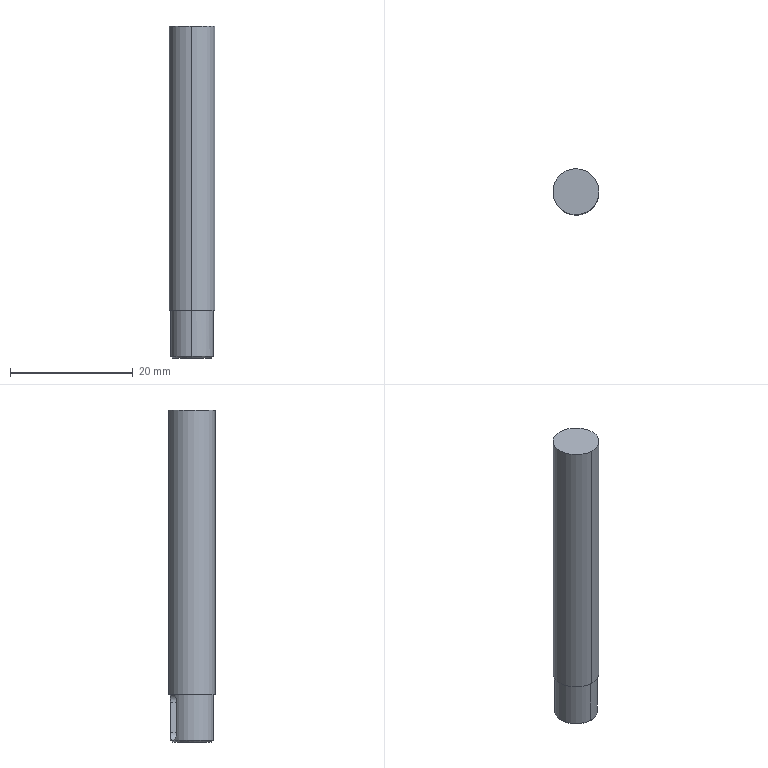Part | STEP file | 2026.6.15-Main Assembly图.sldasm-Part-111 | 1 solid | 20 faces | box 7.5 x 7.5 x 53.995 mm | volume 2283 mm3 | cylinder 9 | plane 7 | cone 4 | commonest cylinder face diameters 2.5 x4 7 x3 7.5 x2
STEP:
#1=CARTESIAN_POINT('',(-1571.384,1420.517,3525.142));
#2=VERTEX_POINT('',#1);
#3=CARTESIAN_POINT('',(-1571.092,1428.011,3525.142));
#4=VERTEX_POINT('',#3);
#5=CARTESIAN_POINT('',(-1571.238,1424.264,3525.142));
#6=DIRECTION('',(0.,0.,1.));
#7=DIRECTION('',(-1.,0.,0.));
#8=AXIS2_PLACEMENT_3D('',#5,#6,#7);
#9=CIRCLE('',#8,3.75);
#10=EDGE_CURVE('',#2,#4,#9,.T.);
#11=ORIENTED_EDGE('',*,*,#10,.F.);
#12=CARTESIAN_POINT('',(-1571.384,1420.517,3478.897));
#13=VERTEX_POINT('',#12);
#14=CARTESIAN_POINT('',(-1571.384,1420.517,3794.147));
#15=DIRECTION('',(0.,0.,-1.));
#16=VECTOR('',#15,1000.);
#17=LINE('',#14,#16);
#18=EDGE_CURVE('',#2,#13,#17,.T.);
#19=ORIENTED_EDGE('',*,*,#18,.T.);
#20=CARTESIAN_POINT('',(-1571.092,1428.011,3478.897));
#21=VERTEX_POINT('',#20);
#22=CARTESIAN_POINT('',(-1571.238,1424.264,3478.897));
#23=DIRECTION('',(0.,0.,1.));
#24=DIRECTION('',(0.03892,0.9992,0.));
#25=AXIS2_PLACEMENT_3D('',#22,#23,#24);
#26=CIRCLE('',#25,3.75);
#27=EDGE_CURVE('',#13,#21,#26,.T.);
#28=ORIENTED_EDGE('',*,*,#27,.T.);
#29=CARTESIAN_POINT('',(-1571.092,1428.011,3794.147));
#30=DIRECTION('',(0.,0.,-1.));
#31=VECTOR('',#30,1000.);
#32=LINE('',#29,#31);
#33=EDGE_CURVE('',#4,#21,#32,.T.);
#34=ORIENTED_EDGE('',*,*,#33,.F.);
#35=EDGE_LOOP('',(#11,#19,#28,#34));
#36=FACE_OUTER_BOUND('',#35,.T.);
#37=CARTESIAN_POINT('',(-1571.238,1424.264,3794.147));
#38=DIRECTION('',(0.,0.,-1.));
#39=DIRECTION('',(0.03892,0.9992,0.));
#40=AXIS2_PLACEMENT_3D('',#37,#38,#39);
#41=CYLINDRICAL_SURFACE('',#40,3.75);
#42=ADVANCED_FACE('',(#36),#41,.T.);
#43=CARTESIAN_POINT('',(-1571.102,1427.762,3478.897));
#44=VERTEX_POINT('',#43);
#45=CARTESIAN_POINT('',(-1571.374,1420.767,3478.897));
#46=VERTEX_POINT('',#45);
#47=CARTESIAN_POINT('',(-1571.238,1424.264,3478.897));
#48=DIRECTION('',(0.,0.,-1.));
#49=DIRECTION('',(0.03892,0.9992,0.));
#50=AXIS2_PLACEMENT_3D('',#47,#48,#49);
#51=CIRCLE('',#50,3.5);
#52=EDGE_CURVE('',#44,#46,#51,.T.);
#53=ORIENTED_EDGE('',*,*,#52,.T.);
#54=CARTESIAN_POINT('',(-1571.374,1420.767,3471.397));
#55=VERTEX_POINT('',#54);
#56=CARTESIAN_POINT('',(-1571.374,1420.767,3478.897));
#57=DIRECTION('',(0.,0.,-1.));
#58=VECTOR('',#57,1000.);
#59=LINE('',#56,#58);
#60=EDGE_CURVE('',#46,#55,#59,.T.);
#61=ORIENTED_EDGE('',*,*,#60,.T.);
#62=CARTESIAN_POINT('',(-1571.241,1420.764,3471.397));
#63=VERTEX_POINT('',#62);
#64=CARTESIAN_POINT('',(-1571.238,1424.264,3471.397));
#65=DIRECTION('',(0.,0.,1.));
#66=DIRECTION('',(0.0007664,1.,0.));
#67=AXIS2_PLACEMENT_3D('',#64,#65,#66);
#68=CIRCLE('',#67,3.5);
#69=EDGE_CURVE('',#55,#63,#68,.T.);
#70=ORIENTED_EDGE('',*,*,#69,.T.);
#71=CARTESIAN_POINT('',(-1571.102,1427.762,3471.397));
#72=VERTEX_POINT('',#71);
#73=CARTESIAN_POINT('',(-1571.238,1424.264,3471.397));
#74=DIRECTION('',(0.,0.,1.));
#75=DIRECTION('',(0.0007664,1.,0.));
#76=AXIS2_PLACEMENT_3D('',#73,#74,#75);
#77=CIRCLE('',#76,3.5);
#78=EDGE_CURVE('',#63,#72,#77,.T.);
#79=ORIENTED_EDGE('',*,*,#78,.T.);
#80=CARTESIAN_POINT('',(-1571.102,1427.762,3478.897));
#81=DIRECTION('',(0.,0.,-1.));
#82=VECTOR('',#81,1000.);
#83=LINE('',#80,#82);
#84=EDGE_CURVE('',#44,#72,#83,.T.);
#85=ORIENTED_EDGE('',*,*,#84,.F.);
#86=EDGE_LOOP('',(#53,#61,#70,#79,#85));
#87=FACE_OUTER_BOUND('',#86,.T.);
#88=CARTESIAN_POINT('',(-1571.238,1424.264,3478.897));
#89=DIRECTION('',(0.,0.,-1.));
#90=DIRECTION('',(0.03892,0.9992,0.));
#91=AXIS2_PLACEMENT_3D('',#88,#89,#90);
#92=CYLINDRICAL_SURFACE('',#91,3.5);
#93=ADVANCED_FACE('',(#87),#92,.T.);
#94=CARTESIAN_POINT('',(-1572.724,1427.433,3478.897));
#95=VERTEX_POINT('',#94);
#96=CARTESIAN_POINT('',(-1571.238,1424.264,3478.897));
#97=DIRECTION('',(0.,0.,-1.));
#98=DIRECTION('',(0.03892,0.9992,0.));
#99=AXIS2_PLACEMENT_3D('',#96,#97,#98);
#100=CIRCLE('',#99,3.5);
#101=EDGE_CURVE('',#95,#44,#100,.T.);
#102=ORIENTED_EDGE('',*,*,#101,.T.);
#103=ORIENTED_EDGE('',*,*,#84,.T.);
#104=CARTESIAN_POINT('',(-1571.236,1427.764,3471.397));
#105=VERTEX_POINT('',#104);
#106=CARTESIAN_POINT('',(-1571.238,1424.264,3471.397));
#107=DIRECTION('',(0.,0.,1.));
#108=DIRECTION('',(0.0007664,1.,0.));
#109=AXIS2_PLACEMENT_3D('',#106,#107,#108);
#110=CIRCLE('',#109,3.5);
#111=EDGE_CURVE('',#72,#105,#110,.T.);
#112=ORIENTED_EDGE('',*,*,#111,.T.);
#113=CARTESIAN_POINT('',(-1572.724,1427.433,3471.397));
#114=VERTEX_POINT('',#113);
#115=CARTESIAN_POINT('',(-1571.238,1424.264,3471.397));
#116=DIRECTION('',(0.,0.,1.));
#117=DIRECTION('',(0.0007664,1.,0.));
#118=AXIS2_PLACEMENT_3D('',#115,#116,#117);
#119=CIRCLE('',#118,3.5);
#120=EDGE_CURVE('',#105,#114,#119,.T.);
#121=ORIENTED_EDGE('',*,*,#120,.T.);
#122=CARTESIAN_POINT('',(-1571.494,1427.755,3472.647));
#123=VERTEX_POINT('',#122);
#124=CARTESIAN_POINT('',(-1571.494,1427.755,3472.647));
#125=CARTESIAN_POINT('',(-1571.494,1427.755,3472.48));
#126=CARTESIAN_POINT('',(-1571.53,1427.753,3472.317));
#127=CARTESIAN_POINT('',(-1571.662,1427.739,3472.015));
#128=CARTESIAN_POINT('',(-1571.759,1427.727,3471.877));
#129=CARTESIAN_POINT('',(-1571.992,1427.684,3471.648));
#130=CARTESIAN_POINT('',(-1572.13,1427.652,3471.555));
#131=CARTESIAN_POINT('',(-1572.419,1427.562,3471.43));
#132=CARTESIAN_POINT('',(-1572.575,1427.503,3471.397));
#133=CARTESIAN_POINT('',(-1572.724,1427.433,3471.397));
#134=B_SPLINE_CURVE_WITH_KNOTS('',3,(#124,#125,#126,#127,#128,#129,#130,#131,#132,#133),.UNSPECIFIED.,.F.,.F.,(4,2,2,2,4),(0.,0.0004927,0.0009855,0.001478,0.001971),.UNSPECIFIED.);
#135=EDGE_CURVE('',#123,#114,#134,.T.);
#136=ORIENTED_EDGE('',*,*,#135,.F.);
#137=CARTESIAN_POINT('',(-1571.494,1427.755,3477.647));
#138=VERTEX_POINT('',#137);
#139=CARTESIAN_POINT('',(-1571.494,1427.755,3478.897));
#140=DIRECTION('',(0.,0.,1.));
#141=VECTOR('',#140,1000.);
#142=LINE('',#139,#141);
#143=EDGE_CURVE('',#123,#138,#142,.T.);
#144=ORIENTED_EDGE('',*,*,#143,.T.);
#145=CARTESIAN_POINT('',(-1572.724,1427.433,3478.897));
#146=CARTESIAN_POINT('',(-1572.649,1427.468,3478.897));
#147=CARTESIAN_POINT('',(-1572.572,1427.501,3478.889));
#148=CARTESIAN_POINT('',(-1572.422,1427.559,3478.856));
#149=CARTESIAN_POINT('',(-1572.348,1427.585,3478.832));
#150=CARTESIAN_POINT('',(-1572.128,1427.653,3478.737));
#151=CARTESIAN_POINT('',(-1571.991,1427.684,3478.645));
#152=CARTESIAN_POINT('',(-1571.817,1427.717,3478.473));
#153=CARTESIAN_POINT('',(-1571.764,1427.725,3478.411));
#154=CARTESIAN_POINT('',(-1571.67,1427.738,3478.276));
#155=CARTESIAN_POINT('',(-1571.629,1427.743,3478.203));
#156=CARTESIAN_POINT('',(-1571.53,1427.753,3477.978));
#157=CARTESIAN_POINT('',(-1571.494,1427.755,3477.813));
#158=CARTESIAN_POINT('',(-1571.494,1427.755,3477.647));
#159=B_SPLINE_CURVE_WITH_KNOTS('',3,(#145,#146,#147,#148,#149,#150,#151,#152,#153,#154,#155,#156,#157,#158),.UNSPECIFIED.,.F.,.F.,(4,2,2,2,2,2,4),(0.001971,0.002217,0.002463,0.002955,0.003201,0.003447,0.003939),.UNSPECIFIED.);
#160=EDGE_CURVE('',#95,#138,#159,.T.);
#161=ORIENTED_EDGE('',*,*,#160,.F.);
#162=EDGE_LOOP('',(#102,#103,#112,#121,#136,#144,#161));
#163=FACE_OUTER_BOUND('',#162,.T.);
#164=CARTESIAN_POINT('',(-1571.238,1424.264,3478.897));
#165=DIRECTION('',(0.,0.,-1.));
#166=DIRECTION('',(0.03892,0.9992,0.));
#167=AXIS2_PLACEMENT_3D('',#164,#165,#166);
#168=CYLINDRICAL_SURFACE('',#167,3.5);
#169=ADVANCED_FACE('',(#163),#168,.T.);
#170=CARTESIAN_POINT('',(-1571.236,1427.514,3471.147));
#171=VERTEX_POINT('',#170);
#172=CARTESIAN_POINT('',(-1571.241,1421.014,3471.147));
#173=VERTEX_POINT('',#172);
#174=CARTESIAN_POINT('',(-1571.238,1424.264,3471.147));
#175=DIRECTION('',(0.,0.,-1.));
#176=DIRECTION('',(0.0007664,1.,0.));
#177=AXIS2_PLACEMENT_3D('',#174,#175,#176);
#178=CIRCLE('',#177,3.25);
#179=EDGE_CURVE('',#171,#173,#178,.T.);
#180=ORIENTED_EDGE('',*,*,#179,.F.);
#181=CARTESIAN_POINT('',(-1571.236,1427.764,3471.397));
#182=DIRECTION('',(0.000542,0.7071,0.7071));
#183=VECTOR('',#182,1000.);
#184=LINE('',#181,#183);
#185=EDGE_CURVE('',#171,#105,#184,.T.);
#186=ORIENTED_EDGE('',*,*,#185,.T.);
#187=ORIENTED_EDGE('',*,*,#111,.F.);
#188=ORIENTED_EDGE('',*,*,#78,.F.);
#189=CARTESIAN_POINT('',(-1571.241,1420.764,3471.397));
#190=DIRECTION('',(-0.000542,-0.7071,0.7071));
#191=VECTOR('',#190,1000.);
#192=LINE('',#189,#191);
#193=EDGE_CURVE('',#173,#63,#192,.T.);
#194=ORIENTED_EDGE('',*,*,#193,.F.);
#195=EDGE_LOOP('',(#180,#186,#187,#188,#194));
#196=FACE_OUTER_BOUND('',#195,.T.);
#197=CARTESIAN_POINT('',(-1571.238,1424.264,3471.397));
#198=DIRECTION('',(0.,0.,1.));
#199=DIRECTION('',(-0.0007664,-1.,0.));
#200=AXIS2_PLACEMENT_3D('',#197,#198,#199);
#201=CONICAL_SURFACE('',#200,3.5,0.7854);
#202=ADVANCED_FACE('',(#196),#201,.T.);
#203=CARTESIAN_POINT('',(-1571.239,1423.014,3471.397));
#204=VERTEX_POINT('',#203);
#205=CARTESIAN_POINT('',(-1571.237,1425.514,3471.397));
#206=VERTEX_POINT('',#205);
#207=CARTESIAN_POINT('',(-1571.238,1424.264,3471.397));
#208=DIRECTION('',(0.,0.,-1.));
#209=DIRECTION('',(0.0007664,1.,0.));
#210=AXIS2_PLACEMENT_3D('',#207,#208,#209);
#211=CIRCLE('',#210,1.25);
#212=EDGE_CURVE('',#204,#206,#211,.T.);
#213=ORIENTED_EDGE('',*,*,#212,.F.);
#214=CARTESIAN_POINT('',(-1571.239,1422.764,3471.147));
#215=VERTEX_POINT('',#214);
#216=CARTESIAN_POINT('',(-1571.239,1422.764,3471.147));
#217=DIRECTION('',(-0.000542,-0.7071,-0.7071));
#218=VECTOR('',#217,1000.);
#219=LINE('',#216,#218);
#220=EDGE_CURVE('',#204,#215,#219,.T.);
#221=ORIENTED_EDGE('',*,*,#220,.T.);
#222=CARTESIAN_POINT('',(-1571.237,1425.764,3471.147));
#223=VERTEX_POINT('',#222);
#224=CARTESIAN_POINT('',(-1571.238,1424.264,3471.147));
#225=DIRECTION('',(0.,0.,1.));
#226=DIRECTION('',(0.0007664,1.,0.));
#227=AXIS2_PLACEMENT_3D('',#224,#225,#226);
#228=CIRCLE('',#227,1.5);
#229=EDGE_CURVE('',#223,#215,#228,.T.);
#230=ORIENTED_EDGE('',*,*,#229,.F.);
#231=CARTESIAN_POINT('',(-1571.237,1425.764,3471.147));
#232=DIRECTION('',(0.000542,0.7071,-0.7071));
#233=VECTOR('',#232,1000.);
#234=LINE('',#231,#233);
#235=EDGE_CURVE('',#206,#223,#234,.T.);
#236=ORIENTED_EDGE('',*,*,#235,.F.);
#237=EDGE_LOOP('',(#213,#221,#230,#236));
#238=FACE_OUTER_BOUND('',#237,.T.);
#239=CARTESIAN_POINT('',(-1571.238,1424.264,3471.147));
#240=DIRECTION('',(0.,0.,-1.));
#241=DIRECTION('',(0.0007664,1.,0.));
#242=AXIS2_PLACEMENT_3D('',#239,#240,#241);
#243=CONICAL_SURFACE('',#242,1.5,0.7854);
#244=ADVANCED_FACE('',(#238),#243,.F.);
#245=ORIENTED_EDGE('',*,*,#212,.T.);
#246=CARTESIAN_POINT('',(-1571.237,1425.514,3478.647));
#247=VERTEX_POINT('',#246);
#248=CARTESIAN_POINT('',(-1571.237,1425.514,3471.147));
#249=DIRECTION('',(0.,0.,1.));
#250=VECTOR('',#249,1000.);
#251=LINE('',#248,#250);
#252=EDGE_CURVE('',#206,#247,#251,.T.);
#253=ORIENTED_EDGE('',*,*,#252,.T.);
#254=CARTESIAN_POINT('',(-1571.239,1423.014,3478.647));
#255=VERTEX_POINT('',#254);
#256=CARTESIAN_POINT('',(-1571.238,1424.264,3478.647));
#257=DIRECTION('',(0.,0.,-1.));
#258=DIRECTION('',(-0.0007664,-1.,0.));
#259=AXIS2_PLACEMENT_3D('',#256,#257,#258);
#260=CIRCLE('',#259,1.25);
#261=EDGE_CURVE('',#255,#247,#260,.T.);
#262=ORIENTED_EDGE('',*,*,#261,.F.);
#263=CARTESIAN_POINT('',(-1571.239,1423.014,3471.147));
#264=DIRECTION('',(0.,0.,1.));
#265=VECTOR('',#264,1000.);
#266=LINE('',#263,#265);
#267=EDGE_CURVE('',#204,#255,#266,.T.);
#268=ORIENTED_EDGE('',*,*,#267,.F.);
#269=EDGE_LOOP('',(#245,#253,#262,#268));
#270=FACE_OUTER_BOUND('',#269,.T.);
#271=CARTESIAN_POINT('',(-1571.238,1424.264,3471.147));
#272=DIRECTION('',(0.,0.,1.));
#273=DIRECTION('',(-0.0007664,-1.,0.));
#274=AXIS2_PLACEMENT_3D('',#271,#272,#273);
#275=CYLINDRICAL_SURFACE('',#274,1.25);
#276=ADVANCED_FACE('',(#270),#275,.F.);
#277=ORIENTED_EDGE('',*,*,#261,.T.);
#278=CARTESIAN_POINT('',(-1571.238,1424.264,3478.647));
#279=DIRECTION('',(0.,0.,-1.));
#280=DIRECTION('',(-0.0007664,-1.,0.));
#281=AXIS2_PLACEMENT_3D('',#278,#279,#280);
#282=CIRCLE('',#281,1.25);
#283=EDGE_CURVE('',#247,#255,#282,.T.);
#284=ORIENTED_EDGE('',*,*,#283,.T.);
#285=EDGE_LOOP('',(#277,#284));
#286=FACE_OUTER_BOUND('',#285,.T.);
#287=CARTESIAN_POINT('',(-1571.238,1424.264,3478.647));
#288=DIRECTION('',(0.,0.,1.));
#289=DIRECTION('',(-0.0007664,-1.,0.));
#290=AXIS2_PLACEMENT_3D('',#287,#288,#289);
#291=PLANE('',#290);
#292=ADVANCED_FACE('',(#286),#291,.F.);
#293=ORIENTED_EDGE('',*,*,#252,.F.);
#294=CARTESIAN_POINT('',(-1571.238,1424.264,3471.397));
#295=DIRECTION('',(0.,0.,-1.));
#296=DIRECTION('',(0.0007664,1.,0.));
#297=AXIS2_PLACEMENT_3D('',#294,#295,#296);
#298=CIRCLE('',#297,1.25);
#299=EDGE_CURVE('',#206,#204,#298,.T.);
#300=ORIENTED_EDGE('',*,*,#299,.T.);
#301=ORIENTED_EDGE('',*,*,#267,.T.);
#302=ORIENTED_EDGE('',*,*,#283,.F.);
#303=EDGE_LOOP('',(#293,#300,#301,#302));
#304=FACE_OUTER_BOUND('',#303,.T.);
#305=CARTESIAN_POINT('',(-1571.238,1424.264,3471.147));
#306=DIRECTION('',(0.,0.,1.));
#307=DIRECTION('',(-0.0007664,-1.,0.));
#308=AXIS2_PLACEMENT_3D('',#305,#306,#307);
#309=CYLINDRICAL_SURFACE('',#308,1.25);
#310=ADVANCED_FACE('',(#304),#309,.F.);
#311=ORIENTED_EDGE('',*,*,#220,.F.);
#312=ORIENTED_EDGE('',*,*,#299,.F.);
#313=ORIENTED_EDGE('',*,*,#235,.T.);
#314=CARTESIAN_POINT('',(-1571.238,1424.264,3471.147));
#315=DIRECTION('',(0.,0.,1.));
#316=DIRECTION('',(0.0007664,1.,0.));
#317=AXIS2_PLACEMENT_3D('',#314,#315,#316);
#318=CIRCLE('',#317,1.5);
#319=EDGE_CURVE('',#215,#223,#318,.T.);
#320=ORIENTED_EDGE('',*,*,#319,.F.);
#321=EDGE_LOOP('',(#311,#312,#313,#320));
#322=FACE_OUTER_BOUND('',#321,.T.);
#323=CARTESIAN_POINT('',(-1571.238,1424.264,3471.147));
#324=DIRECTION('',(0.,0.,-1.));
#325=DIRECTION('',(0.0007664,1.,0.));
#326=AXIS2_PLACEMENT_3D('',#323,#324,#325);
#327=CONICAL_SURFACE('',#326,1.5,0.7854);
#328=ADVANCED_FACE('',(#322),#327,.F.);
#329=ORIENTED_EDGE('',*,*,#229,.T.);
#330=ORIENTED_EDGE('',*,*,#319,.T.);
#331=EDGE_LOOP('',(#329,#330));
#332=FACE_BOUND('',#331,.T.);
#333=CARTESIAN_POINT('',(-1571.238,1424.264,3471.147));
#334=DIRECTION('',(0.,0.,-1.));
#335=DIRECTION('',(0.0007664,1.,0.));
#336=AXIS2_PLACEMENT_3D('',#333,#334,#335);
#337=CIRCLE('',#336,3.25);
#338=EDGE_CURVE('',#173,#171,#337,.T.);
#339=ORIENTED_EDGE('',*,*,#338,.T.);
#340=ORIENTED_EDGE('',*,*,#179,.T.);
#341=EDGE_LOOP('',(#339,#340));
#342=FACE_OUTER_BOUND('',#341,.T.);
#343=CARTESIAN_POINT('',(-1571.238,1424.264,3471.147));
#344=DIRECTION('',(0.,0.,-1.));
#345=DIRECTION('',(0.0007664,1.,0.));
#346=AXIS2_PLACEMENT_3D('',#343,#344,#345);
#347=PLANE('',#346);
#348=ADVANCED_FACE('',(#332,#342),#347,.T.);
#349=CARTESIAN_POINT('',(-1571.061,1426.832,3472.647));
#350=VERTEX_POINT('',#349);
#351=CARTESIAN_POINT('',(-1573.325,1425.771,3472.647));
#352=VERTEX_POINT('',#351);
#353=CARTESIAN_POINT('',(-1572.193,1426.302,3472.647));
#354=DIRECTION('',(-0.4244,0.9055,0.));
#355=DIRECTION('',(0.9052,0.4243,0.02473));
#356=AXIS2_PLACEMENT_3D('',#353,#354,#355);
#357=CIRCLE('',#356,1.25);
#358=EDGE_CURVE('',#350,#352,#357,.T.);
#359=ORIENTED_EDGE('',*,*,#358,.T.);
#360=CARTESIAN_POINT('',(-1573.325,1425.771,3477.647));
#361=VERTEX_POINT('',#360);
#362=CARTESIAN_POINT('',(-1573.325,1425.771,3478.897));
#363=DIRECTION('',(0.,0.,-1.));
#364=VECTOR('',#363,1000.);
#365=LINE('',#362,#364);
#366=EDGE_CURVE('',#361,#352,#365,.T.);
#367=ORIENTED_EDGE('',*,*,#366,.F.);
#368=CARTESIAN_POINT('',(-1571.061,1426.832,3477.647));
#369=VERTEX_POINT('',#368);
#370=CARTESIAN_POINT('',(-1572.193,1426.302,3477.647));
#371=DIRECTION('',(-0.4244,0.9055,0.));
#372=DIRECTION('',(0.9052,0.4243,0.02473));
#373=AXIS2_PLACEMENT_3D('',#370,#371,#372);
#374=CIRCLE('',#373,1.25);
#375=EDGE_CURVE('',#361,#369,#374,.T.);
#376=ORIENTED_EDGE('',*,*,#375,.T.);
#377=CARTESIAN_POINT('',(-1571.061,1426.832,3478.897));
#378=DIRECTION('',(0.,0.,-1.));
#379=VECTOR('',#378,1000.);
#380=LINE('',#377,#379);
#381=EDGE_CURVE('',#369,#350,#380,.T.);
#382=ORIENTED_EDGE('',*,*,#381,.T.);
#383=EDGE_LOOP('',(#359,#367,#376,#382));
#384=FACE_OUTER_BOUND('',#383,.T.);
#385=CARTESIAN_POINT('',(-1573.325,1425.771,3478.897));
#386=DIRECTION('',(0.4244,-0.9055,0.));
#387=DIRECTION('',(0.9052,0.4243,0.02473));
#388=AXIS2_PLACEMENT_3D('',#385,#386,#387);
#389=PLANE('',#388);
#390=ADVANCED_FACE('',(#384),#389,.F.);
#391=ORIENTED_EDGE('',*,*,#185,.F.);
#392=ORIENTED_EDGE('',*,*,#338,.F.);
#393=ORIENTED_EDGE('',*,*,#193,.T.);
#394=ORIENTED_EDGE('',*,*,#69,.F.);
#395=CARTESIAN_POINT('',(-1571.238,1424.264,3471.397));
#396=DIRECTION('',(0.,0.,1.));
#397=DIRECTION('',(0.0007664,1.,0.));
#398=AXIS2_PLACEMENT_3D('',#395,#396,#397);
#399=CIRCLE('',#398,3.5);
#400=EDGE_CURVE('',#114,#55,#399,.T.);
#401=ORIENTED_EDGE('',*,*,#400,.F.);
#402=ORIENTED_EDGE('',*,*,#120,.F.);
#403=EDGE_LOOP('',(#391,#392,#393,#394,#401,#402));
#404=FACE_OUTER_BOUND('',#403,.T.);
#405=CARTESIAN_POINT('',(-1571.238,1424.264,3471.397));
#406=DIRECTION('',(0.,0.,1.));
#407=DIRECTION('',(-0.0007664,-1.,0.));
#408=AXIS2_PLACEMENT_3D('',#405,#406,#407);
#409=CONICAL_SURFACE('',#408,3.5,0.7854);
#410=ADVANCED_FACE('',(#404),#409,.T.);
#411=CARTESIAN_POINT('',(-1573.758,1426.694,3477.647));
#412=VERTEX_POINT('',#411);
#413=CARTESIAN_POINT('',(-1573.325,1425.771,3477.647));
#414=DIRECTION('',(0.4244,-0.9055,0.));
#415=VECTOR('',#414,1000.);
#416=LINE('',#413,#415);
#417=EDGE_CURVE('',#412,#361,#416,.T.);
#418=ORIENTED_EDGE('',*,*,#417,.T.);
#419=ORIENTED_EDGE('',*,*,#366,.T.);
#420=CARTESIAN_POINT('',(-1573.758,1426.694,3472.647));
#421=VERTEX_POINT('',#420);
#422=CARTESIAN_POINT('',(-1573.325,1425.771,3472.647));
#423=DIRECTION('',(-0.4244,0.9055,0.));
#424=VECTOR('',#423,1000.);
#425=LINE('',#422,#424);
#426=EDGE_CURVE('',#352,#421,#425,.T.);
#427=ORIENTED_EDGE('',*,*,#426,.T.);
#428=CARTESIAN_POINT('',(-1573.758,1426.694,3478.897));
#429=DIRECTION('',(0.,0.,-1.));
#430=VECTOR('',#429,1000.);
#431=LINE('',#428,#430);
#432=EDGE_CURVE('',#412,#421,#431,.T.);
#433=ORIENTED_EDGE('',*,*,#432,.F.);
#434=EDGE_LOOP('',(#418,#419,#427,#433));
#435=FACE_OUTER_BOUND('',#434,.T.);
#436=CARTESIAN_POINT('',(-1573.325,1425.771,3478.897));
#437=DIRECTION('',(-0.9055,-0.4244,0.));
#438=DIRECTION('',(0.,0.,-1.));
#439=AXIS2_PLACEMENT_3D('',#436,#437,#438);
#440=PLANE('',#439);
#441=ADVANCED_FACE('',(#435),#440,.F.);
#442=CARTESIAN_POINT('',(-1573.758,1426.694,3477.647));
#443=CARTESIAN_POINT('',(-1573.758,1426.694,3477.814));
#444=CARTESIAN_POINT('',(-1573.733,1426.72,3477.977));
#445=CARTESIAN_POINT('',(-1573.638,1426.813,3478.279));
#446=CARTESIAN_POINT('',(-1573.567,1426.88,3478.417));
#447=CARTESIAN_POINT('',(-1573.385,1427.031,3478.645));
#448=CARTESIAN_POINT('',(-1573.272,1427.117,3478.738));
#449=CARTESIAN_POINT('',(-1573.017,1427.282,3478.863));
#450=CARTESIAN_POINT('',(-1572.873,1427.364,3478.897));
#451=CARTESIAN_POINT('',(-1572.724,1427.433,3478.897));
#452=B_SPLINE_CURVE_WITH_KNOTS('',3,(#442,#443,#444,#445,#446,#447,#448,#449,#450,#451),.UNSPECIFIED.,.F.,.F.,(4,2,2,2,4),(0.,0.0004927,0.0009855,0.001478,0.001971),.UNSPECIFIED.);
#453=EDGE_CURVE('',#412,#95,#452,.T.);
#454=ORIENTED_EDGE('',*,*,#453,.T.);
#455=ORIENTED_EDGE('',*,*,#160,.T.);
#456=CARTESIAN_POINT('',(-1571.061,1426.832,3477.647));
#457=DIRECTION('',(-0.4244,0.9055,0.));
#458=VECTOR('',#457,1000.);
#459=LINE('',#456,#458);
#460=EDGE_CURVE('',#369,#138,#459,.T.);
#461=ORIENTED_EDGE('',*,*,#460,.F.);
#462=ORIENTED_EDGE('',*,*,#375,.F.);
#463=ORIENTED_EDGE('',*,*,#417,.F.);
#464=EDGE_LOOP('',(#454,#455,#461,#462,#463));
#465=FACE_OUTER_BOUND('',#464,.T.);
#466=CARTESIAN_POINT('',(-1572.193,1426.302,3477.647));
#467=DIRECTION('',(-0.4244,0.9055,0.));
#468=DIRECTION('',(-0.9052,-0.4243,-0.02473));
#469=AXIS2_PLACEMENT_3D('',#466,#467,#468);
#470=CYLINDRICAL_SURFACE('',#469,1.25);
#471=ADVANCED_FACE('',(#465),#470,.F.);
#472=CARTESIAN_POINT('',(-1571.061,1426.832,3472.647));
#473=DIRECTION('',(0.4244,-0.9055,0.));
#474=VECTOR('',#473,1000.);
#475=LINE('',#472,#474);
#476=EDGE_CURVE('',#123,#350,#475,.T.);
#477=ORIENTED_EDGE('',*,*,#476,.T.);
#478=ORIENTED_EDGE('',*,*,#381,.F.);
#479=ORIENTED_EDGE('',*,*,#460,.T.);
#480=ORIENTED_EDGE('',*,*,#143,.F.);
#481=EDGE_LOOP('',(#477,#478,#479,#480));
#482=FACE_OUTER_BOUND('',#481,.T.);
#483=CARTESIAN_POINT('',(-1571.061,1426.832,3478.897));
#484=DIRECTION('',(-0.9055,-0.4244,0.));
#485=DIRECTION('',(0.,0.,-1.));
#486=AXIS2_PLACEMENT_3D('',#483,#484,#485);
#487=PLANE('',#486);
#488=ADVANCED_FACE('',(#482),#487,.T.);
#489=ORIENTED_EDGE('',*,*,#135,.T.);
#490=CARTESIAN_POINT('',(-1572.724,1427.433,3471.397));
#491=CARTESIAN_POINT('',(-1572.798,1427.399,3471.397));
#492=CARTESIAN_POINT('',(-1572.873,1427.36,3471.405));
#493=CARTESIAN_POINT('',(-1573.013,1427.282,3471.437));
#494=CARTESIAN_POINT('',(-1573.081,1427.241,3471.461));
#495=CARTESIAN_POINT('',(-1573.274,1427.116,3471.556));
#496=CARTESIAN_POINT('',(-1573.385,1427.031,3471.649));
#497=CARTESIAN_POINT('',(-1573.522,1426.917,3471.821));
#498=CARTESIAN_POINT('',(-1573.562,1426.882,3471.883));
#499=CARTESIAN_POINT('',(-1573.632,1426.818,3472.018));
#500=CARTESIAN_POINT('',(-1573.662,1426.79,3472.091));
#501=CARTESIAN_POINT('',(-1573.733,1426.72,3472.316));
#502=CARTESIAN_POINT('',(-1573.758,1426.694,3472.48));
#503=CARTESIAN_POINT('',(-1573.758,1426.694,3472.647));
#504=B_SPLINE_CURVE_WITH_KNOTS('',3,(#490,#491,#492,#493,#494,#495,#496,#497,#498,#499,#500,#501,#502,#503),.UNSPECIFIED.,.F.,.F.,(4,2,2,2,2,2,4),(0.001971,0.002217,0.002463,0.002955,0.003201,0.003447,0.003939),.UNSPECIFIED.);
#505=EDGE_CURVE('',#114,#421,#504,.T.);
#506=ORIENTED_EDGE('',*,*,#505,.T.);
#507=ORIENTED_EDGE('',*,*,#426,.F.);
#508=ORIENTED_EDGE('',*,*,#358,.F.);
#509=ORIENTED_EDGE('',*,*,#476,.F.);
#510=EDGE_LOOP('',(#489,#506,#507,#508,#509));
#511=FACE_OUTER_BOUND('',#510,.T.);
#512=CARTESIAN_POINT('',(-1572.193,1426.302,3472.647));
#513=DIRECTION('',(0.4244,-0.9055,0.));
#514=DIRECTION('',(0.9052,0.4243,0.02473));
#515=AXIS2_PLACEMENT_3D('',#512,#513,#514);
#516=CYLINDRICAL_SURFACE('',#515,1.25);
#517=ADVANCED_FACE('',(#511),#516,.F.);
#518=ORIENTED_EDGE('',*,*,#60,.F.);
#519=CARTESIAN_POINT('',(-1571.238,1424.264,3478.897));
#520=DIRECTION('',(0.,0.,-1.));
#521=DIRECTION('',(0.03892,0.9992,0.));
#522=AXIS2_PLACEMENT_3D('',#519,#520,#521);
#523=CIRCLE('',#522,3.5);
#524=EDGE_CURVE('',#46,#95,#523,.T.);
#525=ORIENTED_EDGE('',*,*,#524,.T.);
#526=ORIENTED_EDGE('',*,*,#453,.F.);
#527=ORIENTED_EDGE('',*,*,#432,.T.);
#528=ORIENTED_EDGE('',*,*,#505,.F.);
#529=ORIENTED_EDGE('',*,*,#400,.T.);
#530=EDGE_LOOP('',(#518,#525,#526,#527,#528,#529));
#531=FACE_OUTER_BOUND('',#530,.T.);
#532=CARTESIAN_POINT('',(-1571.238,1424.264,3478.897));
#533=DIRECTION('',(0.,0.,-1.));
#534=DIRECTION('',(0.03892,0.9992,0.));
#535=AXIS2_PLACEMENT_3D('',#532,#533,#534);
#536=CYLINDRICAL_SURFACE('',#535,3.5);
#537=ADVANCED_FACE('',(#531),#536,.T.);
#538=CARTESIAN_POINT('',(-1571.238,1424.264,3478.897));
#539=DIRECTION('',(0.,0.,1.));
#540=DIRECTION('',(0.03892,0.9992,0.));
#541=AXIS2_PLACEMENT_3D('',#538,#539,#540);
#542=CIRCLE('',#541,3.75);
#543=EDGE_CURVE('',#21,#13,#542,.T.);
#544=ORIENTED_EDGE('',*,*,#543,.F.);
#545=ORIENTED_EDGE('',*,*,#27,.F.);
#546=EDGE_LOOP('',(#544,#545));
#547=FACE_OUTER_BOUND('',#546,.T.);
#548=ORIENTED_EDGE('',*,*,#101,.F.);
#549=ORIENTED_EDGE('',*,*,#524,.F.);
#550=ORIENTED_EDGE('',*,*,#52,.F.);
#551=EDGE_LOOP('',(#548,#549,#550));
#552=FACE_BOUND('',#551,.T.);
#553=CARTESIAN_POINT('',(-1571.238,1424.264,3478.897));
#554=DIRECTION('',(0.,0.,-1.));
#555=DIRECTION('',(0.0007664,1.,0.));
#556=AXIS2_PLACEMENT_3D('',#553,#554,#555);
#557=PLANE('',#556);
#558=ADVANCED_FACE('',(#547,#552),#557,.T.);
#559=ORIENTED_EDGE('',*,*,#18,.F.);
#560=CARTESIAN_POINT('',(-1571.238,1424.264,3525.142));
#561=DIRECTION('',(0.,0.,1.));
#562=DIRECTION('',(-1.,0.,0.));
#563=AXIS2_PLACEMENT_3D('',#560,#561,#562);
#564=CIRCLE('',#563,3.75);
#565=EDGE_CURVE('',#4,#2,#564,.T.);
#566=ORIENTED_EDGE('',*,*,#565,.F.);
#567=ORIENTED_EDGE('',*,*,#33,.T.);
#568=ORIENTED_EDGE('',*,*,#543,.T.);
#569=EDGE_LOOP('',(#559,#566,#567,#568));
#570=FACE_OUTER_BOUND('',#569,.T.);
#571=CARTESIAN_POINT('',(-1571.238,1424.264,3794.147));
#572=DIRECTION('',(0.,0.,-1.));
#573=DIRECTION('',(0.03892,0.9992,0.));
#574=AXIS2_PLACEMENT_3D('',#571,#572,#573);
#575=CYLINDRICAL_SURFACE('',#574,3.75);
#576=ADVANCED_FACE('',(#570),#575,.T.);
#577=ORIENTED_EDGE('',*,*,#565,.T.);
#578=ORIENTED_EDGE('',*,*,#10,.T.);
#579=EDGE_LOOP('',(#577,#578));
#580=FACE_OUTER_BOUND('',#579,.T.);
#581=CARTESIAN_POINT('',(-1556.42,1410.832,3525.142));
#582=DIRECTION('',(0.,0.,-1.));
#583=DIRECTION('',(-1.,0.,0.));
#584=AXIS2_PLACEMENT_3D('',#581,#582,#583);
#585=PLANE('',#584);
#586=ADVANCED_FACE('',(#580),#585,.F.);
#587=CLOSED_SHELL('',(#42,#93,#169,#202,#244,#276,#292,#310,#328,#348,#390,#410,#441,#471,#488,#517,#537,#558,#576,#586));
#588=MANIFOLD_SOLID_BREP('',#587);
#589=CARTESIAN_POINT('',(0.,0.,0.));
#590=DIRECTION('',(0.,0.,1.));
#591=DIRECTION('',(1.,0.,0.));
#592=AXIS2_PLACEMENT_3D('',#589,#590,#591);
#593=(LENGTH_UNIT()NAMED_UNIT(*)SI_UNIT(.MILLI.,.METRE.));
#594=UNCERTAINTY_MEASURE_WITH_UNIT(LENGTH_MEASURE(0.00001),#593,'','');
#595=(NAMED_UNIT(*)PLANE_ANGLE_UNIT()SI_UNIT($,.RADIAN.));
#596=(NAMED_UNIT(*)SI_UNIT($,.STERADIAN.)SOLID_ANGLE_UNIT());
#597=(GEOMETRIC_REPRESENTATION_CONTEXT(3)GLOBAL_UNCERTAINTY_ASSIGNED_CONTEXT((#594))GLOBAL_UNIT_ASSIGNED_CONTEXT((#593,#595,#596))REPRESENTATION_CONTEXT('',''));
#598=ADVANCED_BREP_SHAPE_REPRESENTATION('',(#588,#592),#597);